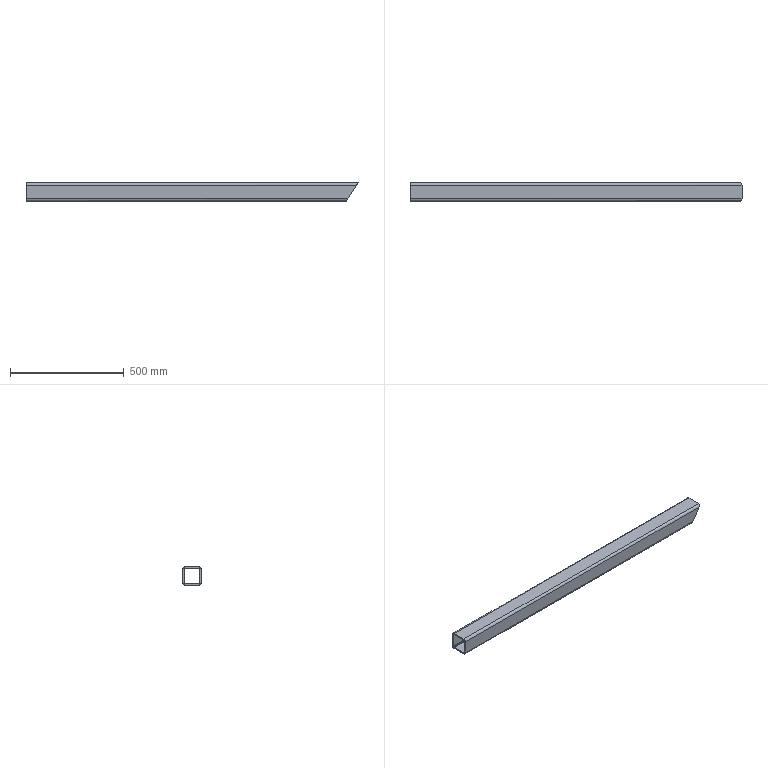Part | NX | features BREP 1 | 1 solid | 39 faces | box 1462 x 80 x 80 mm | volume 2438141 mm3 | cylinder 22 | plane 17 | commonest cylinder face diameters 20 x14 8 x8